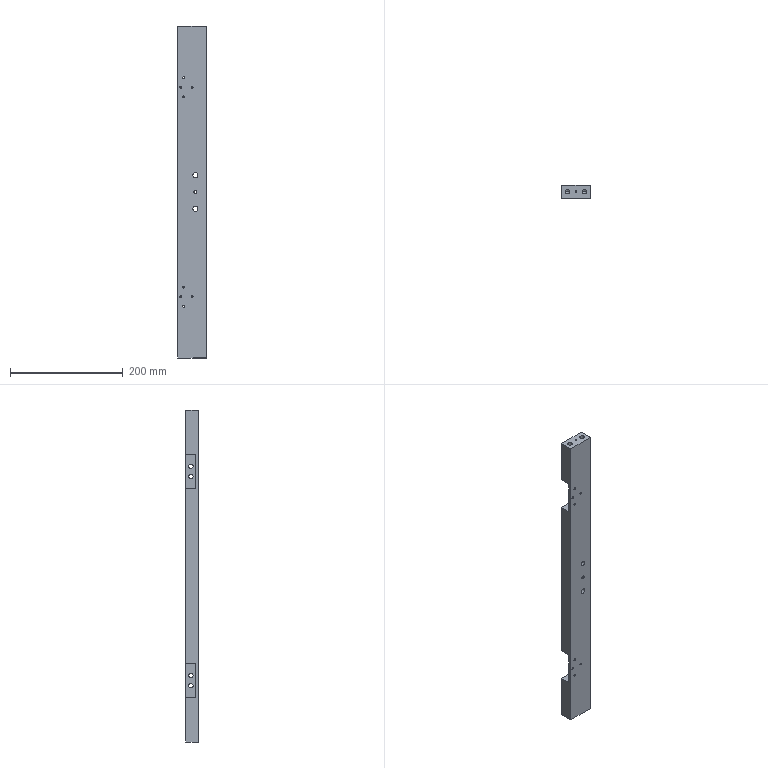Part | SolidWorks | features 3DProfileFeature 4, HoleWzd 4, MirrorPattern 4, Cut 3, ICE 3, Extrusion 1 | 1 solid | 65 faces | box 49.8 x 23 x 590 mm | volume 566573 mm3 | cylinder 42 | plane 17 | cone 6 | commonest cylinder face diameters 3.4 x16 8 x12 9 x4 15 x4 3 x2 5.5 x2